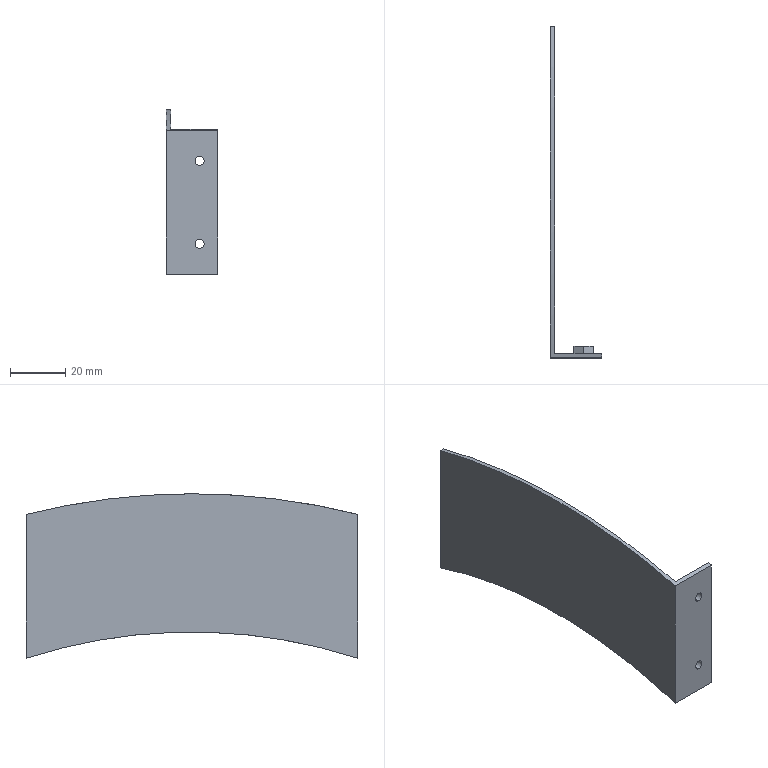Part | STEP file | 09-40 Infeed pressure plate | 1 solid | 26 faces | box 18.5 x 120 x 59.46 mm | volume 10592 mm3 | plane 20 | cylinder 6 | commonest cylinder face diameters 3.3 x4 390 x1 490 x1